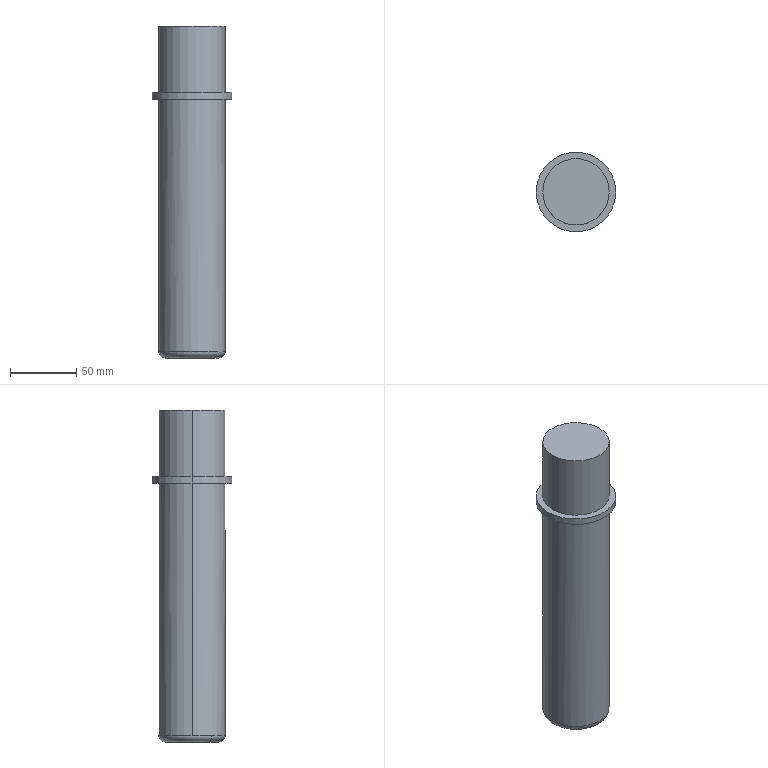Part | 1 solid | 12 faces | box 60 x 60 x 250 mm | volume 494388 mm3 | cylinder 6 | plane 4 | torus 2 | commonest cylinder face diameters 50 x4 60 x2
STEP:
#1=CARTESIAN_POINT('',(0.,0.,0.));
#2=DIRECTION('',(0.,0.,1.));
#3=DIRECTION('',(1.,0.,0.));
#4=AXIS2_PLACEMENT_3D('',#1,#2,#3);
#5=CARTESIAN_POINT('',(-505.,-18.5,-258.051));
#6=VERTEX_POINT('',#5);
#7=CARTESIAN_POINT('',(-505.,-18.5,-68.051));
#8=VERTEX_POINT('',#7);
#9=CARTESIAN_POINT('',(-505.,-18.5,-258.051));
#10=DIRECTION('',(0.,0.,1.));
#11=VECTOR('',#10,1.);
#12=LINE('',#9,#11);
#13=CARTESIAN_POINT('',(-480.,-18.5,-263.051));
#14=DIRECTION('',(0.,0.,1.));
#15=DIRECTION('',(0.,1.,0.));
#16=AXIS2_PLACEMENT_3D('',#13,#14,#15);
#17=CYLINDRICAL_SURFACE('',#16,25.);
#18=CARTESIAN_POINT('',(1.571,5.));
#19=DIRECTION('',(0.,1.));
#20=VECTOR('',#19,1.);
#21=LINE('',#18,#20);
#22=(GEOMETRIC_REPRESENTATION_CONTEXT(2)PARAMETRIC_REPRESENTATION_CONTEXT()REPRESENTATION_CONTEXT('',''));
#23=DEFINITIONAL_REPRESENTATION('',(#21),#22);
#24=PCURVE('',#17,#23);
#25=CARTESIAN_POINT('',(-480.,-18.5,-263.051));
#26=DIRECTION('',(0.,0.,1.));
#27=DIRECTION('',(0.,-1.,0.));
#28=AXIS2_PLACEMENT_3D('',#25,#26,#27);
#29=CYLINDRICAL_SURFACE('',#28,25.);
#30=CARTESIAN_POINT('',(4.712,5.));
#31=DIRECTION('',(0.,1.));
#32=VECTOR('',#31,1.);
#33=LINE('',#30,#32);
#34=(GEOMETRIC_REPRESENTATION_CONTEXT(2)PARAMETRIC_REPRESENTATION_CONTEXT()REPRESENTATION_CONTEXT('',''));
#35=DEFINITIONAL_REPRESENTATION('',(#33),#34);
#36=PCURVE('',#29,#35);
#37=SURFACE_CURVE('',#12,(#24,#36),.PCURVE_S1.);
#38=EDGE_CURVE('',#6,#8,#37,.T.);
#39=ORIENTED_EDGE('',*,*,#38,.F.);
#40=CARTESIAN_POINT('',(-500.225,-33.195,-258.051));
#41=VERTEX_POINT('',#40);
#42=CARTESIAN_POINT('',(-480.,-18.5,-258.051));
#43=DIRECTION('',(0.,0.,1.));
#44=DIRECTION('',(-1.,0.,0.));
#45=AXIS2_PLACEMENT_3D('',#42,#43,#44);
#46=CIRCLE('',#45,25.);
#47=CARTESIAN_POINT('',(1.571,5.));
#48=DIRECTION('',(1.,0.));
#49=VECTOR('',#48,1.);
#50=LINE('',#47,#49);
#51=(GEOMETRIC_REPRESENTATION_CONTEXT(2)PARAMETRIC_REPRESENTATION_CONTEXT()REPRESENTATION_CONTEXT('',''));
#52=DEFINITIONAL_REPRESENTATION('',(#50),#51);
#53=PCURVE('',#17,#52);
#54=CARTESIAN_POINT('',(-480.,-18.5,-258.051));
#55=DIRECTION('',(0.,0.,-1.));
#56=DIRECTION('',(0.5878,-0.809,0.));
#57=AXIS2_PLACEMENT_3D('',#54,#55,#56);
#58=TOROIDAL_SURFACE('',#57,20.,5.);
#59=CARTESIAN_POINT('',(2.199,0.));
#60=DIRECTION('',(-1.,0.));
#61=VECTOR('',#60,1.);
#62=LINE('',#59,#61);
#63=(GEOMETRIC_REPRESENTATION_CONTEXT(2)PARAMETRIC_REPRESENTATION_CONTEXT()REPRESENTATION_CONTEXT('',''));
#64=DEFINITIONAL_REPRESENTATION('',(#62),#63);
#65=PCURVE('',#58,#64);
#66=SURFACE_CURVE('',#46,(#53,#65),.PCURVE_S1.);
#67=EDGE_CURVE('',#6,#41,#66,.T.);
#68=ORIENTED_EDGE('',*,*,#67,.T.);
#69=CARTESIAN_POINT('',(-455.,-18.5,-258.051));
#70=VERTEX_POINT('',#69);
#71=CARTESIAN_POINT('',(-480.,-18.5,-258.051));
#72=DIRECTION('',(0.,0.,1.));
#73=DIRECTION('',(-1.,0.,0.));
#74=AXIS2_PLACEMENT_3D('',#71,#72,#73);
#75=CIRCLE('',#74,25.);
#76=CARTESIAN_POINT('',(1.571,5.));
#77=DIRECTION('',(1.,0.));
#78=VECTOR('',#77,1.);
#79=LINE('',#76,#78);
#80=(GEOMETRIC_REPRESENTATION_CONTEXT(2)PARAMETRIC_REPRESENTATION_CONTEXT()REPRESENTATION_CONTEXT('',''));
#81=DEFINITIONAL_REPRESENTATION('',(#79),#80);
#82=PCURVE('',#17,#81);
#83=CARTESIAN_POINT('',(-480.,-18.5,-258.051));
#84=DIRECTION('',(0.,0.,-1.));
#85=DIRECTION('',(-0.5878,0.809,0.));
#86=AXIS2_PLACEMENT_3D('',#83,#84,#85);
#87=TOROIDAL_SURFACE('',#86,20.,5.);
#88=CARTESIAN_POINT('',(5.341,0.));
#89=DIRECTION('',(-1.,0.));
#90=VECTOR('',#89,1.);
#91=LINE('',#88,#90);
#92=(GEOMETRIC_REPRESENTATION_CONTEXT(2)PARAMETRIC_REPRESENTATION_CONTEXT()REPRESENTATION_CONTEXT('',''));
#93=DEFINITIONAL_REPRESENTATION('',(#91),#92);
#94=PCURVE('',#87,#93);
#95=SURFACE_CURVE('',#75,(#82,#94),.PCURVE_S1.);
#96=EDGE_CURVE('',#41,#70,#95,.T.);
#97=ORIENTED_EDGE('',*,*,#96,.T.);
#98=CARTESIAN_POINT('',(-455.,-18.5,-68.051));
#99=VERTEX_POINT('',#98);
#100=CARTESIAN_POINT('',(-455.,-18.5,-258.051));
#101=DIRECTION('',(0.,0.,1.));
#102=VECTOR('',#101,1.);
#103=LINE('',#100,#102);
#104=CARTESIAN_POINT('',(4.712,5.));
#105=DIRECTION('',(0.,1.));
#106=VECTOR('',#105,1.);
#107=LINE('',#104,#106);
#108=(GEOMETRIC_REPRESENTATION_CONTEXT(2)PARAMETRIC_REPRESENTATION_CONTEXT()REPRESENTATION_CONTEXT('',''));
#109=DEFINITIONAL_REPRESENTATION('',(#107),#108);
#110=PCURVE('',#17,#109);
#111=CARTESIAN_POINT('',(1.571,5.));
#112=DIRECTION('',(0.,1.));
#113=VECTOR('',#112,1.);
#114=LINE('',#111,#113);
#115=(GEOMETRIC_REPRESENTATION_CONTEXT(2)PARAMETRIC_REPRESENTATION_CONTEXT()REPRESENTATION_CONTEXT('',''));
#116=DEFINITIONAL_REPRESENTATION('',(#114),#115);
#117=PCURVE('',#29,#116);
#118=SURFACE_CURVE('',#103,(#110,#117),.PCURVE_S1.);
#119=EDGE_CURVE('',#70,#99,#118,.T.);
#120=ORIENTED_EDGE('',*,*,#119,.T.);
#121=CARTESIAN_POINT('',(-480.,-18.5,-68.051));
#122=DIRECTION('',(0.,0.,1.));
#123=DIRECTION('',(1.,0.,0.));
#124=AXIS2_PLACEMENT_3D('',#121,#122,#123);
#125=CIRCLE('',#124,25.);
#126=CARTESIAN_POINT('',(-1.571,195.));
#127=DIRECTION('',(1.,0.));
#128=VECTOR('',#127,1.);
#129=LINE('',#126,#128);
#130=(GEOMETRIC_REPRESENTATION_CONTEXT(2)PARAMETRIC_REPRESENTATION_CONTEXT()REPRESENTATION_CONTEXT('',''));
#131=DEFINITIONAL_REPRESENTATION('',(#129),#130);
#132=PCURVE('',#17,#131);
#133=CARTESIAN_POINT('',(-480.,-18.5,-68.051));
#134=DIRECTION('',(0.,0.,1.));
#135=DIRECTION('',(1.,0.,0.));
#136=AXIS2_PLACEMENT_3D('',#133,#134,#135);
#137=PLANE('',#136);
#138=CARTESIAN_POINT('',(0.,0.));
#139=DIRECTION('',(1.,0.));
#140=AXIS2_PLACEMENT_2D('',#138,#139);
#141=CIRCLE('',#140,25.);
#142=(GEOMETRIC_REPRESENTATION_CONTEXT(2)PARAMETRIC_REPRESENTATION_CONTEXT()REPRESENTATION_CONTEXT('',''));
#143=DEFINITIONAL_REPRESENTATION('',(#141),#142);
#144=PCURVE('',#137,#143);
#145=SURFACE_CURVE('',#125,(#132,#144),.PCURVE_S1.);
#146=EDGE_CURVE('',#8,#99,#145,.T.);
#147=ORIENTED_EDGE('',*,*,#146,.F.);
#148=EDGE_LOOP('',(#39,#68,#97,#120,#147));
#149=FACE_BOUND('',#148,.T.);
#150=ADVANCED_FACE('',(#149),#17,.T.);
#151=CARTESIAN_POINT('',(-463.82,-6.744,-263.051));
#152=VERTEX_POINT('',#151);
#153=CARTESIAN_POINT('',(-459.775,-3.805,-258.051));
#154=VERTEX_POINT('',#153);
#155=CARTESIAN_POINT('',(-463.82,-6.744,-258.051));
#156=DIRECTION('',(0.5878,-0.809,0.));
#157=DIRECTION('',(0.,0.,-1.));
#158=AXIS2_PLACEMENT_3D('',#155,#156,#157);
#159=CIRCLE('',#158,5.);
#160=CARTESIAN_POINT('',(1.571,1.571));
#161=DIRECTION('',(0.,-1.));
#162=VECTOR('',#161,1.);
#163=LINE('',#160,#162);
#164=(GEOMETRIC_REPRESENTATION_CONTEXT(2)PARAMETRIC_REPRESENTATION_CONTEXT()REPRESENTATION_CONTEXT('',''));
#165=DEFINITIONAL_REPRESENTATION('',(#163),#164);
#166=PCURVE('',#87,#165);
#167=CARTESIAN_POINT('',(4.712,1.571));
#168=DIRECTION('',(0.,-1.));
#169=VECTOR('',#168,1.);
#170=LINE('',#167,#169);
#171=(GEOMETRIC_REPRESENTATION_CONTEXT(2)PARAMETRIC_REPRESENTATION_CONTEXT()REPRESENTATION_CONTEXT('',''));
#172=DEFINITIONAL_REPRESENTATION('',(#170),#171);
#173=PCURVE('',#58,#172);
#174=SURFACE_CURVE('',#159,(#166,#173),.PCURVE_S1.);
#175=EDGE_CURVE('',#152,#154,#174,.T.);
#176=ORIENTED_EDGE('',*,*,#175,.T.);
#177=CARTESIAN_POINT('',(-480.,-18.5,-258.051));
#178=DIRECTION('',(0.,0.,1.));
#179=DIRECTION('',(-1.,0.,0.));
#180=AXIS2_PLACEMENT_3D('',#177,#178,#179);
#181=CIRCLE('',#180,25.);
#182=CARTESIAN_POINT('',(5.341,0.));
#183=DIRECTION('',(-1.,0.));
#184=VECTOR('',#183,1.);
#185=LINE('',#182,#184);
#186=(GEOMETRIC_REPRESENTATION_CONTEXT(2)PARAMETRIC_REPRESENTATION_CONTEXT()REPRESENTATION_CONTEXT('',''));
#187=DEFINITIONAL_REPRESENTATION('',(#185),#186);
#188=PCURVE('',#87,#187);
#189=CARTESIAN_POINT('',(-1.571,5.));
#190=DIRECTION('',(1.,0.));
#191=VECTOR('',#190,1.);
#192=LINE('',#189,#191);
#193=(GEOMETRIC_REPRESENTATION_CONTEXT(2)PARAMETRIC_REPRESENTATION_CONTEXT()REPRESENTATION_CONTEXT('',''));
#194=DEFINITIONAL_REPRESENTATION('',(#192),#193);
#195=PCURVE('',#29,#194);
#196=SURFACE_CURVE('',#181,(#188,#195),.PCURVE_S1.);
#197=EDGE_CURVE('',#70,#154,#196,.T.);
#198=ORIENTED_EDGE('',*,*,#197,.F.);
#199=ORIENTED_EDGE('',*,*,#96,.F.);
#200=CARTESIAN_POINT('',(-496.18,-30.256,-263.051));
#201=VERTEX_POINT('',#200);
#202=CARTESIAN_POINT('',(-496.18,-30.256,-258.051));
#203=DIRECTION('',(-0.5878,0.809,0.));
#204=DIRECTION('',(0.,0.,-1.));
#205=AXIS2_PLACEMENT_3D('',#202,#203,#204);
#206=CIRCLE('',#205,5.);
#207=CARTESIAN_POINT('',(4.712,1.571));
#208=DIRECTION('',(0.,-1.));
#209=VECTOR('',#208,1.);
#210=LINE('',#207,#209);
#211=(GEOMETRIC_REPRESENTATION_CONTEXT(2)PARAMETRIC_REPRESENTATION_CONTEXT()REPRESENTATION_CONTEXT('',''));
#212=DEFINITIONAL_REPRESENTATION('',(#210),#211);
#213=PCURVE('',#87,#212);
#214=CARTESIAN_POINT('',(1.571,1.571));
#215=DIRECTION('',(0.,-1.));
#216=VECTOR('',#215,1.);
#217=LINE('',#214,#216);
#218=(GEOMETRIC_REPRESENTATION_CONTEXT(2)PARAMETRIC_REPRESENTATION_CONTEXT()REPRESENTATION_CONTEXT('',''));
#219=DEFINITIONAL_REPRESENTATION('',(#217),#218);
#220=PCURVE('',#58,#219);
#221=SURFACE_CURVE('',#206,(#213,#220),.PCURVE_S1.);
#222=EDGE_CURVE('',#201,#41,#221,.T.);
#223=ORIENTED_EDGE('',*,*,#222,.F.);
#224=CARTESIAN_POINT('',(-463.82,-30.256,-263.051));
#225=VERTEX_POINT('',#224);
#226=CARTESIAN_POINT('',(-480.,-18.5,-263.051));
#227=DIRECTION('',(0.,0.,-1.));
#228=DIRECTION('',(0.809,-0.5878,0.));
#229=AXIS2_PLACEMENT_3D('',#226,#227,#228);
#230=CIRCLE('',#229,20.);
#231=CARTESIAN_POINT('',(2.827,1.571));
#232=DIRECTION('',(1.,0.));
#233=VECTOR('',#232,1.);
#234=LINE('',#231,#233);
#235=(GEOMETRIC_REPRESENTATION_CONTEXT(2)PARAMETRIC_REPRESENTATION_CONTEXT()REPRESENTATION_CONTEXT('',''));
#236=DEFINITIONAL_REPRESENTATION('',(#234),#235);
#237=PCURVE('',#87,#236);
#238=CARTESIAN_POINT('',(-480.,-18.5,-263.051));
#239=DIRECTION('',(0.,0.,-1.));
#240=DIRECTION('',(-1.,0.,0.));
#241=AXIS2_PLACEMENT_3D('',#238,#239,#240);
#242=PLANE('',#241);
#243=CARTESIAN_POINT('',(0.,0.));
#244=DIRECTION('',(-0.809,-0.5878));
#245=AXIS2_PLACEMENT_2D('',#243,#244);
#246=CIRCLE('',#245,20.);
#247=(GEOMETRIC_REPRESENTATION_CONTEXT(2)PARAMETRIC_REPRESENTATION_CONTEXT()REPRESENTATION_CONTEXT('',''));
#248=DEFINITIONAL_REPRESENTATION('',(#246),#247);
#249=PCURVE('',#242,#248);
#250=SURFACE_CURVE('',#230,(#237,#249),.PCURVE_S1.);
#251=EDGE_CURVE('',#225,#201,#250,.T.);
#252=ORIENTED_EDGE('',*,*,#251,.F.);
#253=CARTESIAN_POINT('',(-480.,-18.5,-263.051));
#254=DIRECTION('',(0.,0.,-1.));
#255=DIRECTION('',(0.809,-0.5878,0.));
#256=AXIS2_PLACEMENT_3D('',#253,#254,#255);
#257=CIRCLE('',#256,20.);
#258=CARTESIAN_POINT('',(-3.456,1.571));
#259=DIRECTION('',(1.,0.));
#260=VECTOR('',#259,1.);
#261=LINE('',#258,#260);
#262=(GEOMETRIC_REPRESENTATION_CONTEXT(2)PARAMETRIC_REPRESENTATION_CONTEXT()REPRESENTATION_CONTEXT('',''));
#263=DEFINITIONAL_REPRESENTATION('',(#261),#262);
#264=PCURVE('',#87,#263);
#265=CARTESIAN_POINT('',(0.,0.));
#266=DIRECTION('',(-0.809,-0.5878));
#267=AXIS2_PLACEMENT_2D('',#265,#266);
#268=CIRCLE('',#267,20.);
#269=(GEOMETRIC_REPRESENTATION_CONTEXT(2)PARAMETRIC_REPRESENTATION_CONTEXT()REPRESENTATION_CONTEXT('',''));
#270=DEFINITIONAL_REPRESENTATION('',(#268),#269);
#271=PCURVE('',#242,#270);
#272=SURFACE_CURVE('',#257,(#264,#271),.PCURVE_S1.);
#273=EDGE_CURVE('',#152,#225,#272,.T.);
#274=ORIENTED_EDGE('',*,*,#273,.F.);
#275=EDGE_LOOP('',(#176,#198,#199,#223,#252,#274));
#276=FACE_BOUND('',#275,.T.);
#277=ADVANCED_FACE('',(#276),#87,.T.);
#278=ORIENTED_EDGE('',*,*,#251,.T.);
#279=CARTESIAN_POINT('',(-480.,-18.5,-263.051));
#280=DIRECTION('',(0.,0.,-1.));
#281=DIRECTION('',(0.809,-0.5878,0.));
#282=AXIS2_PLACEMENT_3D('',#279,#280,#281);
#283=CIRCLE('',#282,20.);
#284=CARTESIAN_POINT('',(0.,0.));
#285=DIRECTION('',(-0.809,-0.5878));
#286=AXIS2_PLACEMENT_2D('',#284,#285);
#287=CIRCLE('',#286,20.);
#288=(GEOMETRIC_REPRESENTATION_CONTEXT(2)PARAMETRIC_REPRESENTATION_CONTEXT()REPRESENTATION_CONTEXT('',''));
#289=DEFINITIONAL_REPRESENTATION('',(#287),#288);
#290=PCURVE('',#242,#289);
#291=CARTESIAN_POINT('',(-0.3142,1.571));
#292=DIRECTION('',(1.,0.));
#293=VECTOR('',#292,1.);
#294=LINE('',#291,#293);
#295=(GEOMETRIC_REPRESENTATION_CONTEXT(2)PARAMETRIC_REPRESENTATION_CONTEXT()REPRESENTATION_CONTEXT('',''));
#296=DEFINITIONAL_REPRESENTATION('',(#294),#295);
#297=PCURVE('',#58,#296);
#298=SURFACE_CURVE('',#283,(#290,#297),.PCURVE_S1.);
#299=EDGE_CURVE('',#201,#152,#298,.T.);
#300=ORIENTED_EDGE('',*,*,#299,.T.);
#301=ORIENTED_EDGE('',*,*,#273,.T.);
#302=EDGE_LOOP('',(#278,#300,#301));
#303=FACE_BOUND('',#302,.T.);
#304=ADVANCED_FACE('',(#303),#242,.T.);
#305=CARTESIAN_POINT('',(-450.,-18.5,-68.051));
#306=VERTEX_POINT('',#305);
#307=CARTESIAN_POINT('',(-510.,-18.5,-68.051));
#308=VERTEX_POINT('',#307);
#309=CARTESIAN_POINT('',(-480.,-18.5,-68.051));
#310=DIRECTION('',(0.,0.,1.));
#311=DIRECTION('',(-1.,0.,0.));
#312=AXIS2_PLACEMENT_3D('',#309,#310,#311);
#313=CIRCLE('',#312,30.);
#314=CARTESIAN_POINT('',(0.,0.));
#315=DIRECTION('',(-1.,0.));
#316=AXIS2_PLACEMENT_2D('',#314,#315);
#317=CIRCLE('',#316,30.);
#318=(GEOMETRIC_REPRESENTATION_CONTEXT(2)PARAMETRIC_REPRESENTATION_CONTEXT()REPRESENTATION_CONTEXT('',''));
#319=DEFINITIONAL_REPRESENTATION('',(#317),#318);
#320=PCURVE('',#137,#319);
#321=CARTESIAN_POINT('',(-480.,-18.5,-63.051));
#322=DIRECTION('',(0.,0.,-1.));
#323=DIRECTION('',(0.,-1.,0.));
#324=AXIS2_PLACEMENT_3D('',#321,#322,#323);
#325=CYLINDRICAL_SURFACE('',#324,30.);
#326=CARTESIAN_POINT('',(7.854,5.));
#327=DIRECTION('',(-1.,0.));
#328=VECTOR('',#327,1.);
#329=LINE('',#326,#328);
#330=(GEOMETRIC_REPRESENTATION_CONTEXT(2)PARAMETRIC_REPRESENTATION_CONTEXT()REPRESENTATION_CONTEXT('',''));
#331=DEFINITIONAL_REPRESENTATION('',(#329),#330);
#332=PCURVE('',#325,#331);
#333=SURFACE_CURVE('',#313,(#320,#332),.PCURVE_S1.);
#334=EDGE_CURVE('',#306,#308,#333,.T.);
#335=ORIENTED_EDGE('',*,*,#334,.F.);
#336=CARTESIAN_POINT('',(-480.,-18.5,-68.051));
#337=DIRECTION('',(0.,0.,1.));
#338=DIRECTION('',(-1.,0.,0.));
#339=AXIS2_PLACEMENT_3D('',#336,#337,#338);
#340=CIRCLE('',#339,30.);
#341=CARTESIAN_POINT('',(0.,0.));
#342=DIRECTION('',(-1.,0.));
#343=AXIS2_PLACEMENT_2D('',#341,#342);
#344=CIRCLE('',#343,30.);
#345=(GEOMETRIC_REPRESENTATION_CONTEXT(2)PARAMETRIC_REPRESENTATION_CONTEXT()REPRESENTATION_CONTEXT('',''));
#346=DEFINITIONAL_REPRESENTATION('',(#344),#345);
#347=PCURVE('',#137,#346);
#348=CARTESIAN_POINT('',(-480.,-18.5,-63.051));
#349=DIRECTION('',(0.,0.,-1.));
#350=DIRECTION('',(0.,1.,0.));
#351=AXIS2_PLACEMENT_3D('',#348,#349,#350);
#352=CYLINDRICAL_SURFACE('',#351,30.);
#353=CARTESIAN_POINT('',(4.712,5.));
#354=DIRECTION('',(-1.,0.));
#355=VECTOR('',#354,1.);
#356=LINE('',#353,#355);
#357=(GEOMETRIC_REPRESENTATION_CONTEXT(2)PARAMETRIC_REPRESENTATION_CONTEXT()REPRESENTATION_CONTEXT('',''));
#358=DEFINITIONAL_REPRESENTATION('',(#356),#357);
#359=PCURVE('',#352,#358);
#360=SURFACE_CURVE('',#340,(#347,#359),.PCURVE_S1.);
#361=EDGE_CURVE('',#308,#306,#360,.T.);
#362=ORIENTED_EDGE('',*,*,#361,.F.);
#363=EDGE_LOOP('',(#335,#362));
#364=FACE_BOUND('',#363,.T.);
#365=CARTESIAN_POINT('',(-480.,-18.5,-68.051));
#366=DIRECTION('',(0.,0.,1.));
#367=DIRECTION('',(1.,0.,0.));
#368=AXIS2_PLACEMENT_3D('',#365,#366,#367);
#369=CIRCLE('',#368,25.);
#370=CARTESIAN_POINT('',(0.,0.));
#371=DIRECTION('',(1.,0.));
#372=AXIS2_PLACEMENT_2D('',#370,#371);
#373=CIRCLE('',#372,25.);
#374=(GEOMETRIC_REPRESENTATION_CONTEXT(2)PARAMETRIC_REPRESENTATION_CONTEXT()REPRESENTATION_CONTEXT('',''));
#375=DEFINITIONAL_REPRESENTATION('',(#373),#374);
#376=PCURVE('',#137,#375);
#377=CARTESIAN_POINT('',(1.571,195.));
#378=DIRECTION('',(1.,0.));
#379=VECTOR('',#378,1.);
#380=LINE('',#377,#379);
#381=(GEOMETRIC_REPRESENTATION_CONTEXT(2)PARAMETRIC_REPRESENTATION_CONTEXT()REPRESENTATION_CONTEXT('',''));
#382=DEFINITIONAL_REPRESENTATION('',(#380),#381);
#383=PCURVE('',#29,#382);
#384=SURFACE_CURVE('',#369,(#376,#383),.PCURVE_S1.);
#385=EDGE_CURVE('',#99,#8,#384,.T.);
#386=ORIENTED_EDGE('',*,*,#385,.T.);
#387=ORIENTED_EDGE('',*,*,#146,.T.);
#388=EDGE_LOOP('',(#386,#387));
#389=FACE_BOUND('',#388,.T.);
#390=ADVANCED_FACE('',(#364,#389),#137,.F.);
#391=CARTESIAN_POINT('',(-450.,-18.5,-63.051));
#392=VERTEX_POINT('',#391);
#393=CARTESIAN_POINT('',(-450.,-18.5,-63.051));
#394=DIRECTION('',(0.,0.,-1.));
#395=VECTOR('',#394,1.);
#396=LINE('',#393,#395);
#397=CARTESIAN_POINT('',(1.571,0.));
#398=DIRECTION('',(0.,1.));
#399=VECTOR('',#398,1.);
#400=LINE('',#397,#399);
#401=(GEOMETRIC_REPRESENTATION_CONTEXT(2)PARAMETRIC_REPRESENTATION_CONTEXT()REPRESENTATION_CONTEXT('',''));
#402=DEFINITIONAL_REPRESENTATION('',(#400),#401);
#403=PCURVE('',#352,#402);
#404=CARTESIAN_POINT('',(4.712,0.));
#405=DIRECTION('',(0.,1.));
#406=VECTOR('',#405,1.);
#407=LINE('',#404,#406);
#408=(GEOMETRIC_REPRESENTATION_CONTEXT(2)PARAMETRIC_REPRESENTATION_CONTEXT()REPRESENTATION_CONTEXT('',''));
#409=DEFINITIONAL_REPRESENTATION('',(#407),#408);
#410=PCURVE('',#325,#409);
#411=SURFACE_CURVE('',#396,(#403,#410),.PCURVE_S1.);
#412=EDGE_CURVE('',#392,#306,#411,.T.);
#413=ORIENTED_EDGE('',*,*,#412,.F.);
#414=CARTESIAN_POINT('',(-510.,-18.5,-63.051));
#415=VERTEX_POINT('',#414);
#416=CARTESIAN_POINT('',(-480.,-18.5,-63.051));
#417=DIRECTION('',(0.,0.,1.));
#418=DIRECTION('',(-1.,0.,0.));
#419=AXIS2_PLACEMENT_3D('',#416,#417,#418);
#420=CIRCLE('',#419,30.);
#421=CARTESIAN_POINT('',(4.712,0.));
#422=DIRECTION('',(-1.,0.));
#423=VECTOR('',#422,1.);
#424=LINE('',#421,#423);
#425=(GEOMETRIC_REPRESENTATION_CONTEXT(2)PARAMETRIC_REPRESENTATION_CONTEXT()REPRESENTATION_CONTEXT('',''));
#426=DEFINITIONAL_REPRESENTATION('',(#424),#425);
#427=PCURVE('',#352,#426);
#428=CARTESIAN_POINT('',(-480.,-18.5,-63.051));
#429=DIRECTION('',(0.,0.,1.));
#430=DIRECTION('',(1.,0.,0.));
#431=AXIS2_PLACEMENT_3D('',#428,#429,#430);
#432=PLANE('',#431);
#433=CARTESIAN_POINT('',(0.,0.));
#434=DIRECTION('',(-1.,0.));
#435=AXIS2_PLACEMENT_2D('',#433,#434);
#436=CIRCLE('',#435,30.);
#437=(GEOMETRIC_REPRESENTATION_CONTEXT(2)PARAMETRIC_REPRESENTATION_CONTEXT()REPRESENTATION_CONTEXT('',''));
#438=DEFINITIONAL_REPRESENTATION('',(#436),#437);
#439=PCURVE('',#432,#438);
#440=SURFACE_CURVE('',#420,(#427,#439),.PCURVE_S1.);
#441=EDGE_CURVE('',#415,#392,#440,.T.);
#442=ORIENTED_EDGE('',*,*,#441,.F.);
#443=CARTESIAN_POINT('',(-510.,-18.5,-63.051));
#444=DIRECTION('',(0.,0.,-1.));
#445=VECTOR('',#444,1.);
#446=LINE('',#443,#445);
#447=CARTESIAN_POINT('',(4.712,0.));
#448=DIRECTION('',(0.,1.));
#449=VECTOR('',#448,1.);
#450=LINE('',#447,#449);
#451=(GEOMETRIC_REPRESENTATION_CONTEXT(2)PARAMETRIC_REPRESENTATION_CONTEXT()REPRESENTATION_CONTEXT('',''));
#452=DEFINITIONAL_REPRESENTATION('',(#450),#451);
#453=PCURVE('',#352,#452);
#454=CARTESIAN_POINT('',(1.571,0.));
#455=DIRECTION('',(0.,1.));
#456=VECTOR('',#455,1.);
#457=LINE('',#454,#456);
#458=(GEOMETRIC_REPRESENTATION_CONTEXT(2)PARAMETRIC_REPRESENTATION_CONTEXT()REPRESENTATION_CONTEXT('',''));
#459=DEFINITIONAL_REPRESENTATION('',(#457),#458);
#460=PCURVE('',#325,#459);
#461=SURFACE_CURVE('',#446,(#453,#460),.PCURVE_S1.);
#462=EDGE_CURVE('',#415,#308,#461,.T.);
#463=ORIENTED_EDGE('',*,*,#462,.T.);
#464=ORIENTED_EDGE('',*,*,#361,.T.);
#465=EDGE_LOOP('',(#413,#442,#463,#464));
#466=FACE_BOUND('',#465,.T.);
#467=ADVANCED_FACE('',(#466),#352,.T.);
#468=ORIENTED_EDGE('',*,*,#441,.T.);
#469=CARTESIAN_POINT('',(-480.,-18.5,-63.051));
#470=DIRECTION('',(0.,0.,1.));
#471=DIRECTION('',(-1.,0.,0.));
#472=AXIS2_PLACEMENT_3D('',#469,#470,#471);
#473=CIRCLE('',#472,30.);
#474=CARTESIAN_POINT('',(0.,0.));
#475=DIRECTION('',(-1.,0.));
#476=AXIS2_PLACEMENT_2D('',#474,#475);
#477=CIRCLE('',#476,30.);
#478=(GEOMETRIC_REPRESENTATION_CONTEXT(2)PARAMETRIC_REPRESENTATION_CONTEXT()REPRESENTATION_CONTEXT('',''));
#479=DEFINITIONAL_REPRESENTATION('',(#477),#478);
#480=PCURVE('',#432,#479);
#481=CARTESIAN_POINT('',(7.854,0.));
#482=DIRECTION('',(-1.,0.));
#483=VECTOR('',#482,1.);
#484=LINE('',#481,#483);
#485=(GEOMETRIC_REPRESENTATION_CONTEXT(2)PARAMETRIC_REPRESENTATION_CONTEXT()REPRESENTATION_CONTEXT('',''));
#486=DEFINITIONAL_REPRESENTATION('',(#484),#485);
#487=PCURVE('',#325,#486);
#488=SURFACE_CURVE('',#473,(#480,#487),.PCURVE_S1.);
#489=EDGE_CURVE('',#392,#415,#488,.T.);
#490=ORIENTED_EDGE('',*,*,#489,.T.);
#491=EDGE_LOOP('',(#468,#490));
#492=FACE_BOUND('',#491,.T.);
#493=CARTESIAN_POINT('',(-505.,-18.5,-63.051));
#494=VERTEX_POINT('',#493);
#495=CARTESIAN_POINT('',(-455.,-18.5,-63.051));
#496=VERTEX_POINT('',#495);
#497=CARTESIAN_POINT('',(-480.,-18.5,-63.051));
#498=DIRECTION('',(0.,0.,1.));
#499=DIRECTION('',(1.,0.,0.));
#500=AXIS2_PLACEMENT_3D('',#497,#498,#499);
#501=CIRCLE('',#500,25.);
#502=CARTESIAN_POINT('',(0.,0.));
#503=DIRECTION('',(1.,0.));
#504=AXIS2_PLACEMENT_2D('',#502,#503);
#505=CIRCLE('',#504,25.);
#506=(GEOMETRIC_REPRESENTATION_CONTEXT(2)PARAMETRIC_REPRESENTATION_CONTEXT()REPRESENTATION_CONTEXT('',''));
#507=DEFINITIONAL_REPRESENTATION('',(#505),#506);
#508=PCURVE('',#432,#507);
#509=CARTESIAN_POINT('',(-480.,-18.5,-263.051));
#510=DIRECTION('',(0.,0.,1.));
#511=DIRECTION('',(0.,1.,0.));
#512=AXIS2_PLACEMENT_3D('',#509,#510,#511);
#513=CYLINDRICAL_SURFACE('',#512,25.);
#514=CARTESIAN_POINT('',(-1.571,200.));
#515=DIRECTION('',(1.,0.));
#516=VECTOR('',#515,1.);
#517=LINE('',#514,#516);
#518=(GEOMETRIC_REPRESENTATION_CONTEXT(2)PARAMETRIC_REPRESENTATION_CONTEXT()REPRESENTATION_CONTEXT('',''));
#519=DEFINITIONAL_REPRESENTATION('',(#517),#518);
#520=PCURVE('',#513,#519);
#521=SURFACE_CURVE('',#501,(#508,#520),.PCURVE_S1.);
#522=EDGE_CURVE('',#494,#496,#521,.T.);
#523=ORIENTED_EDGE('',*,*,#522,.F.);
#524=CARTESIAN_POINT('',(-480.,-18.5,-63.051));
#525=DIRECTION('',(0.,0.,1.));
#526=DIRECTION('',(1.,0.,0.));
#527=AXIS2_PLACEMENT_3D('',#524,#525,#526);
#528=CIRCLE('',#527,25.);
#529=CARTESIAN_POINT('',(0.,0.));
#530=DIRECTION('',(1.,0.));
#531=AXIS2_PLACEMENT_2D('',#529,#530);
#532=CIRCLE('',#531,25.);
#533=(GEOMETRIC_REPRESENTATION_CONTEXT(2)PARAMETRIC_REPRESENTATION_CONTEXT()REPRESENTATION_CONTEXT('',''));
#534=DEFINITIONAL_REPRESENTATION('',(#532),#533);
#535=PCURVE('',#432,#534);
#536=CARTESIAN_POINT('',(-480.,-18.5,-263.051));
#537=DIRECTION('',(0.,0.,1.));
#538=DIRECTION('',(0.,-1.,0.));
#539=AXIS2_PLACEMENT_3D('',#536,#537,#538);
#540=CYLINDRICAL_SURFACE('',#539,25.);
#541=CARTESIAN_POINT('',(1.571,200.));
#542=DIRECTION('',(1.,0.));
#543=VECTOR('',#542,1.);
#544=LINE('',#541,#543);
#545=(GEOMETRIC_REPRESENTATION_CONTEXT(2)PARAMETRIC_REPRESENTATION_CONTEXT()REPRESENTATION_CONTEXT('',''));
#546=DEFINITIONAL_REPRESENTATION('',(#544),#545);
#547=PCURVE('',#540,#546);
#548=SURFACE_CURVE('',#528,(#535,#547),.PCURVE_S1.);
#549=EDGE_CURVE('',#496,#494,#548,.T.);
#550=ORIENTED_EDGE('',*,*,#549,.F.);
#551=EDGE_LOOP('',(#523,#550));
#552=FACE_BOUND('',#551,.T.);
#553=ADVANCED_FACE('',(#492,#552),#432,.T.);
#554=CARTESIAN_POINT('',(-505.,-18.5,-13.051));
#555=VERTEX_POINT('',#554);
#556=CARTESIAN_POINT('',(-505.,-18.5,-63.051));
#557=DIRECTION('',(0.,0.,1.));
#558=VECTOR('',#557,1.);
#559=LINE('',#556,#558);
#560=CARTESIAN_POINT('',(1.571,200.));
#561=DIRECTION('',(0.,1.));
#562=VECTOR('',#561,1.);
#563=LINE('',#560,#562);
#564=(GEOMETRIC_REPRESENTATION_CONTEXT(2)PARAMETRIC_REPRESENTATION_CONTEXT()REPRESENTATION_CONTEXT('',''));
#565=DEFINITIONAL_REPRESENTATION('',(#563),#564);
#566=PCURVE('',#513,#565);
#567=CARTESIAN_POINT('',(4.712,200.));
#568=DIRECTION('',(0.,1.));
#569=VECTOR('',#568,1.);
#570=LINE('',#567,#569);
#571=(GEOMETRIC_REPRESENTATION_CONTEXT(2)PARAMETRIC_REPRESENTATION_CONTEXT()REPRESENTATION_CONTEXT('',''));
#572=DEFINITIONAL_REPRESENTATION('',(#570),#571);
#573=PCURVE('',#540,#572);
#574=SURFACE_CURVE('',#559,(#566,#573),.PCURVE_S1.);
#575=EDGE_CURVE('',#494,#555,#574,.T.);
#576=ORIENTED_EDGE('',*,*,#575,.F.);
#577=ORIENTED_EDGE('',*,*,#522,.T.);
#578=CARTESIAN_POINT('',(-455.,-18.5,-13.051));
#579=VERTEX_POINT('',#578);
#580=CARTESIAN_POINT('',(-455.,-18.5,-63.051));
#581=DIRECTION('',(0.,0.,1.));
#582=VECTOR('',#581,1.);
#583=LINE('',#580,#582);
#584=CARTESIAN_POINT('',(4.712,200.));
#585=DIRECTION('',(0.,1.));
#586=VECTOR('',#585,1.);
#587=LINE('',#584,#586);
#588=(GEOMETRIC_REPRESENTATION_CONTEXT(2)PARAMETRIC_REPRESENTATION_CONTEXT()REPRESENTATION_CONTEXT('',''));
#589=DEFINITIONAL_REPRESENTATION('',(#587),#588);
#590=PCURVE('',#513,#589);
#591=CARTESIAN_POINT('',(1.571,200.));
#592=DIRECTION('',(0.,1.));
#593=VECTOR('',#592,1.);
#594=LINE('',#591,#593);
#595=(GEOMETRIC_REPRESENTATION_CONTEXT(2)PARAMETRIC_REPRESENTATION_CONTEXT()REPRESENTATION_CONTEXT('',''));
#596=DEFINITIONAL_REPRESENTATION('',(#594),#595);
#597=PCURVE('',#540,#596);
#598=SURFACE_CURVE('',#583,(#590,#597),.PCURVE_S1.);
#599=EDGE_CURVE('',#496,#579,#598,.T.);
#600=ORIENTED_EDGE('',*,*,#599,.T.);
#601=CARTESIAN_POINT('',(-480.,-18.5,-13.051));
#602=DIRECTION('',(0.,0.,1.));
#603=DIRECTION('',(1.,0.,0.));
#604=AXIS2_PLACEMENT_3D('',#601,#602,#603);
#605=CIRCLE('',#604,25.);
#606=CARTESIAN_POINT('',(-1.571,250.));
#607=DIRECTION('',(1.,0.));
#608=VECTOR('',#607,1.);
#609=LINE('',#606,#608);
#610=(GEOMETRIC_REPRESENTATION_CONTEXT(2)PARAMETRIC_REPRESENTATION_CONTEXT()REPRESENTATION_CONTEXT('',''));
#611=DEFINITIONAL_REPRESENTATION('',(#609),#610);
#612=PCURVE('',#513,#611);
#613=CARTESIAN_POINT('',(-480.,-18.5,-13.051));
#614=DIRECTION('',(0.,0.,-1.));
#615=DIRECTION('',(-1.,0.,0.));
#616=AXIS2_PLACEMENT_3D('',#613,#614,#615);
#617=PLANE('',#616);
#618=CARTESIAN_POINT('',(-25.,0.));
#619=CARTESIAN_POINT('',(-25.,43.301));
#620=CARTESIAN_POINT('',(12.5,21.651));
#621=CARTESIAN_POINT('',(50.,0.));
#622=CARTESIAN_POINT('',(12.5,-21.651));
#623=CARTESIAN_POINT('',(-25.,-43.301));
#624=CARTESIAN_POINT('',(-25.,0.));
#625=(BOUNDED_CURVE()B_SPLINE_CURVE(2,(#618,#619,#620,#621,#622,#623,#624),.UNSPECIFIED.,.T.,.F.)B_SPLINE_CURVE_WITH_KNOTS((1,2,2,2,2,1),(-2.094,0.,2.094,4.189,6.283,8.378),.UNSPECIFIED.)CURVE()GEOMETRIC_REPRESENTATION_ITEM()RATIONAL_B_SPLINE_CURVE((1.,0.5,1.,0.5,1.,0.5,1.))REPRESENTATION_ITEM(''));
#626=(GEOMETRIC_REPRESENTATION_CONTEXT(2)PARAMETRIC_REPRESENTATION_CONTEXT()REPRESENTATION_CONTEXT('',''));
#627=DEFINITIONAL_REPRESENTATION('',(#625),#626);
#628=PCURVE('',#617,#627);
#629=SURFACE_CURVE('',#605,(#612,#628),.PCURVE_S1.);
#630=EDGE_CURVE('',#555,#579,#629,.T.);
#631=ORIENTED_EDGE('',*,*,#630,.F.);
#632=EDGE_LOOP('',(#576,#577,#600,#631));
#633=FACE_BOUND('',#632,.T.);
#634=ADVANCED_FACE('',(#633),#513,.T.);
#635=CARTESIAN_POINT('',(-480.,-18.5,-13.051));
#636=DIRECTION('',(0.,0.,1.));
#637=DIRECTION('',(1.,0.,0.));
#638=AXIS2_PLACEMENT_3D('',#635,#636,#637);
#639=CIRCLE('',#638,25.);
#640=CARTESIAN_POINT('',(-25.,0.));
#641=CARTESIAN_POINT('',(-25.,43.301));
#642=CARTESIAN_POINT('',(12.5,21.651));
#643=CARTESIAN_POINT('',(50.,0.));
#644=CARTESIAN_POINT('',(12.5,-21.651));
#645=CARTESIAN_POINT('',(-25.,-43.301));
#646=CARTESIAN_POINT('',(-25.,0.));
#647=(BOUNDED_CURVE()B_SPLINE_CURVE(2,(#640,#641,#642,#643,#644,#645,#646),.UNSPECIFIED.,.T.,.F.)B_SPLINE_CURVE_WITH_KNOTS((1,2,2,2,2,1),(-2.094,0.,2.094,4.189,6.283,8.378),.UNSPECIFIED.)CURVE()GEOMETRIC_REPRESENTATION_ITEM()RATIONAL_B_SPLINE_CURVE((1.,0.5,1.,0.5,1.,0.5,1.))REPRESENTATION_ITEM(''));
#648=(GEOMETRIC_REPRESENTATION_CONTEXT(2)PARAMETRIC_REPRESENTATION_CONTEXT()REPRESENTATION_CONTEXT('',''));
#649=DEFINITIONAL_REPRESENTATION('',(#647),#648);
#650=PCURVE('',#617,#649);
#651=CARTESIAN_POINT('',(1.571,250.));
#652=DIRECTION('',(1.,0.));
#653=VECTOR('',#652,1.);
#654=LINE('',#651,#653);
#655=(GEOMETRIC_REPRESENTATION_CONTEXT(2)PARAMETRIC_REPRESENTATION_CONTEXT()REPRESENTATION_CONTEXT('',''));
#656=DEFINITIONAL_REPRESENTATION('',(#654),#655);
#657=PCURVE('',#540,#656);
#658=SURFACE_CURVE('',#639,(#650,#657),.PCURVE_S1.);
#659=EDGE_CURVE('',#579,#555,#658,.T.);
#660=ORIENTED_EDGE('',*,*,#659,.T.);
#661=ORIENTED_EDGE('',*,*,#630,.T.);
#662=EDGE_LOOP('',(#660,#661));
#663=FACE_BOUND('',#662,.T.);
#664=ADVANCED_FACE('',(#663),#617,.F.);
#665=ORIENTED_EDGE('',*,*,#38,.T.);
#666=ORIENTED_EDGE('',*,*,#385,.F.);
#667=ORIENTED_EDGE('',*,*,#119,.F.);
#668=ORIENTED_EDGE('',*,*,#197,.T.);
#669=CARTESIAN_POINT('',(-480.,-18.5,-258.051));
#670=DIRECTION('',(0.,0.,1.));
#671=DIRECTION('',(-1.,0.,0.));
#672=AXIS2_PLACEMENT_3D('',#669,#670,#671);
#673=CIRCLE('',#672,25.);
#674=CARTESIAN_POINT('',(-1.571,5.));
#675=DIRECTION('',(1.,0.));
#676=VECTOR('',#675,1.);
#677=LINE('',#674,#676);
#678=(GEOMETRIC_REPRESENTATION_CONTEXT(2)PARAMETRIC_REPRESENTATION_CONTEXT()REPRESENTATION_CONTEXT('',''));
#679=DEFINITIONAL_REPRESENTATION('',(#677),#678);
#680=PCURVE('',#29,#679);
#681=CARTESIAN_POINT('',(8.482,0.));
#682=DIRECTION('',(-1.,0.));
#683=VECTOR('',#682,1.);
#684=LINE('',#681,#683);
#685=(GEOMETRIC_REPRESENTATION_CONTEXT(2)PARAMETRIC_REPRESENTATION_CONTEXT()REPRESENTATION_CONTEXT('',''));
#686=DEFINITIONAL_REPRESENTATION('',(#684),#685);
#687=PCURVE('',#58,#686);
#688=SURFACE_CURVE('',#673,(#680,#687),.PCURVE_S1.);
#689=EDGE_CURVE('',#154,#6,#688,.T.);
#690=ORIENTED_EDGE('',*,*,#689,.T.);
#691=EDGE_LOOP('',(#665,#666,#667,#668,#690));
#692=FACE_BOUND('',#691,.T.);
#693=ADVANCED_FACE('',(#692),#29,.T.);
#694=ORIENTED_EDGE('',*,*,#175,.F.);
#695=ORIENTED_EDGE('',*,*,#299,.F.);
#696=ORIENTED_EDGE('',*,*,#222,.T.);
#697=ORIENTED_EDGE('',*,*,#67,.F.);
#698=ORIENTED_EDGE('',*,*,#689,.F.);
#699=EDGE_LOOP('',(#694,#695,#696,#697,#698));
#700=FACE_BOUND('',#699,.T.);
#701=ADVANCED_FACE('',(#700),#58,.T.);
#702=ORIENTED_EDGE('',*,*,#412,.T.);
#703=ORIENTED_EDGE('',*,*,#334,.T.);
#704=ORIENTED_EDGE('',*,*,#462,.F.);
#705=ORIENTED_EDGE('',*,*,#489,.F.);
#706=EDGE_LOOP('',(#702,#703,#704,#705));
#707=FACE_BOUND('',#706,.T.);
#708=ADVANCED_FACE('',(#707),#325,.T.);
#709=ORIENTED_EDGE('',*,*,#575,.T.);
#710=ORIENTED_EDGE('',*,*,#659,.F.);
#711=ORIENTED_EDGE('',*,*,#599,.F.);
#712=ORIENTED_EDGE('',*,*,#549,.T.);
#713=EDGE_LOOP('',(#709,#710,#711,#712));
#714=FACE_BOUND('',#713,.T.);
#715=ADVANCED_FACE('',(#714),#540,.T.);
#716=CLOSED_SHELL('',(#150,#277,#304,#390,#467,#553,#634,#664,#693,#701,#708,#715));
#717=MANIFOLD_SOLID_BREP('',#716);
#718=(LENGTH_UNIT()NAMED_UNIT(*)SI_UNIT(.MILLI.,.METRE.));
#719=UNCERTAINTY_MEASURE_WITH_UNIT(LENGTH_MEASURE(0.0000001),#718,'','');
#720=(NAMED_UNIT(*)PLANE_ANGLE_UNIT()SI_UNIT($,.RADIAN.));
#721=(NAMED_UNIT(*)SI_UNIT($,.STERADIAN.)SOLID_ANGLE_UNIT());
#722=(GEOMETRIC_REPRESENTATION_CONTEXT(3)GLOBAL_UNCERTAINTY_ASSIGNED_CONTEXT((#719))GLOBAL_UNIT_ASSIGNED_CONTEXT((#718,#720,#721))REPRESENTATION_CONTEXT('',''));
#723=ADVANCED_BREP_SHAPE_REPRESENTATION('',(#4,#717),#722);